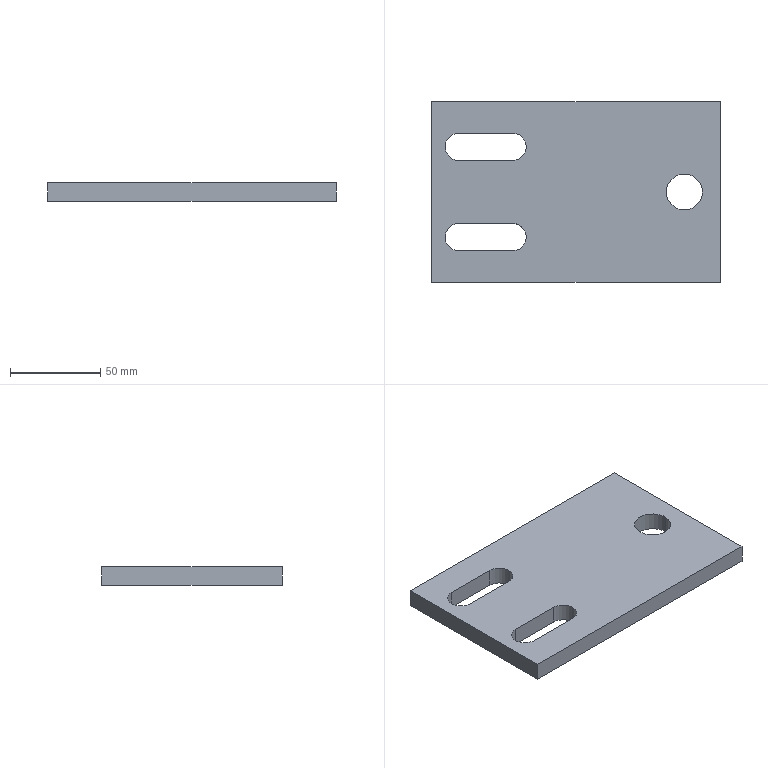Part | SolidWorks | features BaseBody 1 | 1 solid | 18 faces | box 160 x 100 x 10 mm | volume 144324 mm3 | plane 10 | cylinder 8 | commonest cylinder face diameters 15 x6 20 x2
STEP:
#1=CARTESIAN_POINT('',(70.,0.,0.));
#2=VERTEX_POINT('',#1);
#3=CARTESIAN_POINT('',(50.,0.,0.));
#4=VERTEX_POINT('',#3);
#5=CARTESIAN_POINT('',(60.,0.,0.));
#6=DIRECTION('',(0.,0.,-1.));
#7=DIRECTION('',(1.,0.,0.));
#8=AXIS2_PLACEMENT_3D('',#5,#6,#7);
#9=CIRCLE('',#8,10.);
#10=EDGE_CURVE('',#2,#4,#9,.T.);
#11=ORIENTED_EDGE('',*,*,#10,.T.);
#12=CARTESIAN_POINT('',(50.,0.,10.));
#13=VERTEX_POINT('',#12);
#14=CARTESIAN_POINT('',(50.,0.,0.));
#15=DIRECTION('',(0.,0.,1.));
#16=VECTOR('',#15,1000.);
#17=LINE('',#14,#16);
#18=EDGE_CURVE('',#4,#13,#17,.T.);
#19=ORIENTED_EDGE('',*,*,#18,.T.);
#20=CARTESIAN_POINT('',(70.,0.,10.));
#21=VERTEX_POINT('',#20);
#22=CARTESIAN_POINT('',(60.,0.,10.));
#23=DIRECTION('',(0.,0.,-1.));
#24=DIRECTION('',(1.,0.,0.));
#25=AXIS2_PLACEMENT_3D('',#22,#23,#24);
#26=CIRCLE('',#25,10.);
#27=EDGE_CURVE('',#21,#13,#26,.T.);
#28=ORIENTED_EDGE('',*,*,#27,.F.);
#29=CARTESIAN_POINT('',(70.,0.,0.));
#30=DIRECTION('',(0.,0.,1.));
#31=VECTOR('',#30,1000.);
#32=LINE('',#29,#31);
#33=EDGE_CURVE('',#2,#21,#32,.T.);
#34=ORIENTED_EDGE('',*,*,#33,.F.);
#35=EDGE_LOOP('',(#11,#19,#28,#34));
#36=FACE_OUTER_BOUND('',#35,.T.);
#37=CARTESIAN_POINT('',(60.,0.,0.));
#38=DIRECTION('',(0.,0.,1.));
#39=DIRECTION('',(1.,0.,0.));
#40=AXIS2_PLACEMENT_3D('',#37,#38,#39);
#41=CYLINDRICAL_SURFACE('',#40,10.);
#42=ADVANCED_FACE('',(#36),#41,.F.);
#43=CARTESIAN_POINT('',(-72.5,-25.,10.));
#44=VERTEX_POINT('',#43);
#45=CARTESIAN_POINT('',(-65.,-17.5,10.));
#46=VERTEX_POINT('',#45);
#47=CARTESIAN_POINT('',(-65.,-25.,10.));
#48=DIRECTION('',(0.,0.,-1.));
#49=DIRECTION('',(-1.,0.,0.));
#50=AXIS2_PLACEMENT_3D('',#47,#48,#49);
#51=CIRCLE('',#50,7.5);
#52=EDGE_CURVE('',#44,#46,#51,.T.);
#53=ORIENTED_EDGE('',*,*,#52,.F.);
#54=CARTESIAN_POINT('',(-72.5,-25.,0.));
#55=VERTEX_POINT('',#54);
#56=CARTESIAN_POINT('',(-72.5,-25.,10.));
#57=DIRECTION('',(0.,0.,-1.));
#58=VECTOR('',#57,1000.);
#59=LINE('',#56,#58);
#60=EDGE_CURVE('',#44,#55,#59,.T.);
#61=ORIENTED_EDGE('',*,*,#60,.T.);
#62=CARTESIAN_POINT('',(-65.,-17.5,0.));
#63=VERTEX_POINT('',#62);
#64=CARTESIAN_POINT('',(-65.,-25.,0.));
#65=DIRECTION('',(0.,0.,-1.));
#66=DIRECTION('',(-1.,0.,0.));
#67=AXIS2_PLACEMENT_3D('',#64,#65,#66);
#68=CIRCLE('',#67,7.5);
#69=EDGE_CURVE('',#55,#63,#68,.T.);
#70=ORIENTED_EDGE('',*,*,#69,.T.);
#71=CARTESIAN_POINT('',(-65.,-17.5,10.));
#72=DIRECTION('',(0.,0.,1.));
#73=VECTOR('',#72,1000.);
#74=LINE('',#71,#73);
#75=EDGE_CURVE('',#63,#46,#74,.T.);
#76=ORIENTED_EDGE('',*,*,#75,.T.);
#77=EDGE_LOOP('',(#53,#61,#70,#76));
#78=FACE_OUTER_BOUND('',#77,.T.);
#79=CARTESIAN_POINT('',(-65.,-25.,10.));
#80=DIRECTION('',(0.,0.,-1.));
#81=DIRECTION('',(-1.,0.,0.));
#82=AXIS2_PLACEMENT_3D('',#79,#80,#81);
#83=CYLINDRICAL_SURFACE('',#82,7.5);
#84=ADVANCED_FACE('',(#78),#83,.F.);
#85=CARTESIAN_POINT('',(-72.5,25.,10.));
#86=VERTEX_POINT('',#85);
#87=CARTESIAN_POINT('',(-65.,32.5,10.));
#88=VERTEX_POINT('',#87);
#89=CARTESIAN_POINT('',(-65.,25.,10.));
#90=DIRECTION('',(0.,0.,-1.));
#91=DIRECTION('',(-1.,0.,0.));
#92=AXIS2_PLACEMENT_3D('',#89,#90,#91);
#93=CIRCLE('',#92,7.5);
#94=EDGE_CURVE('',#86,#88,#93,.T.);
#95=ORIENTED_EDGE('',*,*,#94,.F.);
#96=CARTESIAN_POINT('',(-72.5,25.,0.));
#97=VERTEX_POINT('',#96);
#98=CARTESIAN_POINT('',(-72.5,25.,10.));
#99=DIRECTION('',(0.,0.,-1.));
#100=VECTOR('',#99,1000.);
#101=LINE('',#98,#100);
#102=EDGE_CURVE('',#86,#97,#101,.T.);
#103=ORIENTED_EDGE('',*,*,#102,.T.);
#104=CARTESIAN_POINT('',(-65.,32.5,0.));
#105=VERTEX_POINT('',#104);
#106=CARTESIAN_POINT('',(-65.,25.,0.));
#107=DIRECTION('',(0.,0.,-1.));
#108=DIRECTION('',(-1.,0.,0.));
#109=AXIS2_PLACEMENT_3D('',#106,#107,#108);
#110=CIRCLE('',#109,7.5);
#111=EDGE_CURVE('',#97,#105,#110,.T.);
#112=ORIENTED_EDGE('',*,*,#111,.T.);
#113=CARTESIAN_POINT('',(-65.,32.5,10.));
#114=DIRECTION('',(0.,0.,1.));
#115=VECTOR('',#114,1000.);
#116=LINE('',#113,#115);
#117=EDGE_CURVE('',#105,#88,#116,.T.);
#118=ORIENTED_EDGE('',*,*,#117,.T.);
#119=EDGE_LOOP('',(#95,#103,#112,#118));
#120=FACE_OUTER_BOUND('',#119,.T.);
#121=CARTESIAN_POINT('',(-65.,25.,10.));
#122=DIRECTION('',(0.,0.,-1.));
#123=DIRECTION('',(-1.,0.,0.));
#124=AXIS2_PLACEMENT_3D('',#121,#122,#123);
#125=CYLINDRICAL_SURFACE('',#124,7.5);
#126=ADVANCED_FACE('',(#120),#125,.F.);
#127=ORIENTED_EDGE('',*,*,#10,.F.);
#128=CARTESIAN_POINT('',(60.,0.,0.));
#129=DIRECTION('',(0.,0.,-1.));
#130=DIRECTION('',(1.,0.,0.));
#131=AXIS2_PLACEMENT_3D('',#128,#129,#130);
#132=CIRCLE('',#131,10.);
#133=EDGE_CURVE('',#4,#2,#132,.T.);
#134=ORIENTED_EDGE('',*,*,#133,.F.);
#135=EDGE_LOOP('',(#127,#134));
#136=FACE_BOUND('',#135,.T.);
#137=CARTESIAN_POINT('',(-35.,-17.5,0.));
#138=VERTEX_POINT('',#137);
#139=CARTESIAN_POINT('',(0.,-17.5,0.));
#140=DIRECTION('',(1.,0.,0.));
#141=VECTOR('',#140,1000.);
#142=LINE('',#139,#141);
#143=EDGE_CURVE('',#63,#138,#142,.T.);
#144=ORIENTED_EDGE('',*,*,#143,.F.);
#145=ORIENTED_EDGE('',*,*,#69,.F.);
#146=CARTESIAN_POINT('',(-65.,-32.5,0.));
#147=VERTEX_POINT('',#146);
#148=CARTESIAN_POINT('',(-65.,-25.,0.));
#149=DIRECTION('',(0.,0.,-1.));
#150=DIRECTION('',(-1.,0.,0.));
#151=AXIS2_PLACEMENT_3D('',#148,#149,#150);
#152=CIRCLE('',#151,7.5);
#153=EDGE_CURVE('',#147,#55,#152,.T.);
#154=ORIENTED_EDGE('',*,*,#153,.F.);
#155=CARTESIAN_POINT('',(-35.,-32.5,0.));
#156=VERTEX_POINT('',#155);
#157=CARTESIAN_POINT('',(0.,-32.5,0.));
#158=DIRECTION('',(-1.,0.,0.));
#159=VECTOR('',#158,1000.);
#160=LINE('',#157,#159);
#161=EDGE_CURVE('',#156,#147,#160,.T.);
#162=ORIENTED_EDGE('',*,*,#161,.F.);
#163=CARTESIAN_POINT('',(-35.,-25.,0.));
#164=DIRECTION('',(0.,0.,-1.));
#165=DIRECTION('',(-1.,0.,0.));
#166=AXIS2_PLACEMENT_3D('',#163,#164,#165);
#167=CIRCLE('',#166,7.5);
#168=EDGE_CURVE('',#138,#156,#167,.T.);
#169=ORIENTED_EDGE('',*,*,#168,.F.);
#170=EDGE_LOOP('',(#144,#145,#154,#162,#169));
#171=FACE_BOUND('',#170,.T.);
#172=CARTESIAN_POINT('',(-35.,32.5,0.));
#173=VERTEX_POINT('',#172);
#174=CARTESIAN_POINT('',(0.,32.5,0.));
#175=DIRECTION('',(1.,0.,0.));
#176=VECTOR('',#175,1000.);
#177=LINE('',#174,#176);
#178=EDGE_CURVE('',#105,#173,#177,.T.);
#179=ORIENTED_EDGE('',*,*,#178,.F.);
#180=ORIENTED_EDGE('',*,*,#111,.F.);
#181=CARTESIAN_POINT('',(-65.,17.5,0.));
#182=VERTEX_POINT('',#181);
#183=CARTESIAN_POINT('',(-65.,25.,0.));
#184=DIRECTION('',(0.,0.,-1.));
#185=DIRECTION('',(-1.,0.,0.));
#186=AXIS2_PLACEMENT_3D('',#183,#184,#185);
#187=CIRCLE('',#186,7.5);
#188=EDGE_CURVE('',#182,#97,#187,.T.);
#189=ORIENTED_EDGE('',*,*,#188,.F.);
#190=CARTESIAN_POINT('',(-35.,17.5,0.));
#191=VERTEX_POINT('',#190);
#192=CARTESIAN_POINT('',(0.,17.5,0.));
#193=DIRECTION('',(-1.,0.,0.));
#194=VECTOR('',#193,1000.);
#195=LINE('',#192,#194);
#196=EDGE_CURVE('',#191,#182,#195,.T.);
#197=ORIENTED_EDGE('',*,*,#196,.F.);
#198=CARTESIAN_POINT('',(-35.,25.,0.));
#199=DIRECTION('',(0.,0.,-1.));
#200=DIRECTION('',(-1.,0.,0.));
#201=AXIS2_PLACEMENT_3D('',#198,#199,#200);
#202=CIRCLE('',#201,7.5);
#203=EDGE_CURVE('',#173,#191,#202,.T.);
#204=ORIENTED_EDGE('',*,*,#203,.F.);
#205=EDGE_LOOP('',(#179,#180,#189,#197,#204));
#206=FACE_BOUND('',#205,.T.);
#207=CARTESIAN_POINT('',(80.,-50.,0.));
#208=VERTEX_POINT('',#207);
#209=CARTESIAN_POINT('',(80.,50.,0.));
#210=VERTEX_POINT('',#209);
#211=CARTESIAN_POINT('',(80.,0.,0.));
#212=DIRECTION('',(0.,1.,0.));
#213=VECTOR('',#212,1000.);
#214=LINE('',#211,#213);
#215=EDGE_CURVE('',#208,#210,#214,.T.);
#216=ORIENTED_EDGE('',*,*,#215,.F.);
#217=CARTESIAN_POINT('',(-80.,-50.,0.));
#218=VERTEX_POINT('',#217);
#219=CARTESIAN_POINT('',(0.,-50.,0.));
#220=DIRECTION('',(1.,0.,0.));
#221=VECTOR('',#220,1000.);
#222=LINE('',#219,#221);
#223=EDGE_CURVE('',#218,#208,#222,.T.);
#224=ORIENTED_EDGE('',*,*,#223,.F.);
#225=CARTESIAN_POINT('',(-80.,50.,0.));
#226=VERTEX_POINT('',#225);
#227=CARTESIAN_POINT('',(-80.,0.,0.));
#228=DIRECTION('',(0.,-1.,0.));
#229=VECTOR('',#228,1000.);
#230=LINE('',#227,#229);
#231=EDGE_CURVE('',#226,#218,#230,.T.);
#232=ORIENTED_EDGE('',*,*,#231,.F.);
#233=CARTESIAN_POINT('',(0.,50.,0.));
#234=DIRECTION('',(-1.,0.,0.));
#235=VECTOR('',#234,1000.);
#236=LINE('',#233,#235);
#237=EDGE_CURVE('',#210,#226,#236,.T.);
#238=ORIENTED_EDGE('',*,*,#237,.F.);
#239=EDGE_LOOP('',(#216,#224,#232,#238));
#240=FACE_OUTER_BOUND('',#239,.T.);
#241=CARTESIAN_POINT('',(0.,0.,0.));
#242=DIRECTION('',(0.,0.,1.));
#243=DIRECTION('',(1.,0.,0.));
#244=AXIS2_PLACEMENT_3D('',#241,#242,#243);
#245=PLANE('',#244);
#246=ADVANCED_FACE('',(#136,#171,#206,#240),#245,.F.);
#247=ORIENTED_EDGE('',*,*,#18,.F.);
#248=ORIENTED_EDGE('',*,*,#133,.T.);
#249=ORIENTED_EDGE('',*,*,#33,.T.);
#250=CARTESIAN_POINT('',(60.,0.,10.));
#251=DIRECTION('',(0.,0.,-1.));
#252=DIRECTION('',(1.,0.,0.));
#253=AXIS2_PLACEMENT_3D('',#250,#251,#252);
#254=CIRCLE('',#253,10.);
#255=EDGE_CURVE('',#13,#21,#254,.T.);
#256=ORIENTED_EDGE('',*,*,#255,.F.);
#257=EDGE_LOOP('',(#247,#248,#249,#256));
#258=FACE_OUTER_BOUND('',#257,.T.);
#259=CARTESIAN_POINT('',(60.,0.,0.));
#260=DIRECTION('',(0.,0.,1.));
#261=DIRECTION('',(1.,0.,0.));
#262=AXIS2_PLACEMENT_3D('',#259,#260,#261);
#263=CYLINDRICAL_SURFACE('',#262,10.);
#264=ADVANCED_FACE('',(#258),#263,.F.);
#265=CARTESIAN_POINT('',(-35.,-17.5,10.));
#266=VERTEX_POINT('',#265);
#267=CARTESIAN_POINT('',(-35.,-17.5,10.));
#268=DIRECTION('',(0.,0.,1.));
#269=VECTOR('',#268,1000.);
#270=LINE('',#267,#269);
#271=EDGE_CURVE('',#138,#266,#270,.T.);
#272=ORIENTED_EDGE('',*,*,#271,.F.);
#273=ORIENTED_EDGE('',*,*,#168,.T.);
#274=CARTESIAN_POINT('',(-35.,-32.5,10.));
#275=VERTEX_POINT('',#274);
#276=CARTESIAN_POINT('',(-35.,-32.5,10.));
#277=DIRECTION('',(0.,0.,-1.));
#278=VECTOR('',#277,1000.);
#279=LINE('',#276,#278);
#280=EDGE_CURVE('',#275,#156,#279,.T.);
#281=ORIENTED_EDGE('',*,*,#280,.F.);
#282=CARTESIAN_POINT('',(-35.,-25.,10.));
#283=DIRECTION('',(0.,0.,-1.));
#284=DIRECTION('',(-1.,0.,0.));
#285=AXIS2_PLACEMENT_3D('',#282,#283,#284);
#286=CIRCLE('',#285,7.5);
#287=EDGE_CURVE('',#266,#275,#286,.T.);
#288=ORIENTED_EDGE('',*,*,#287,.F.);
#289=EDGE_LOOP('',(#272,#273,#281,#288));
#290=FACE_OUTER_BOUND('',#289,.T.);
#291=CARTESIAN_POINT('',(-35.,-25.,10.));
#292=DIRECTION('',(0.,0.,-1.));
#293=DIRECTION('',(-1.,0.,0.));
#294=AXIS2_PLACEMENT_3D('',#291,#292,#293);
#295=CYLINDRICAL_SURFACE('',#294,7.5);
#296=ADVANCED_FACE('',(#290),#295,.F.);
#297=ORIENTED_EDGE('',*,*,#75,.F.);
#298=ORIENTED_EDGE('',*,*,#143,.T.);
#299=ORIENTED_EDGE('',*,*,#271,.T.);
#300=CARTESIAN_POINT('',(-65.,-17.5,10.));
#301=DIRECTION('',(1.,0.,0.));
#302=VECTOR('',#301,1000.);
#303=LINE('',#300,#302);
#304=EDGE_CURVE('',#46,#266,#303,.T.);
#305=ORIENTED_EDGE('',*,*,#304,.F.);
#306=EDGE_LOOP('',(#297,#298,#299,#305));
#307=FACE_OUTER_BOUND('',#306,.T.);
#308=CARTESIAN_POINT('',(-65.,-17.5,10.));
#309=DIRECTION('',(0.,1.,0.));
#310=DIRECTION('',(0.,0.,1.));
#311=AXIS2_PLACEMENT_3D('',#308,#309,#310);
#312=PLANE('',#311);
#313=ADVANCED_FACE('',(#307),#312,.F.);
#314=ORIENTED_EDGE('',*,*,#60,.F.);
#315=CARTESIAN_POINT('',(-65.,-32.5,10.));
#316=VERTEX_POINT('',#315);
#317=CARTESIAN_POINT('',(-65.,-25.,10.));
#318=DIRECTION('',(0.,0.,-1.));
#319=DIRECTION('',(-1.,0.,0.));
#320=AXIS2_PLACEMENT_3D('',#317,#318,#319);
#321=CIRCLE('',#320,7.5);
#322=EDGE_CURVE('',#316,#44,#321,.T.);
#323=ORIENTED_EDGE('',*,*,#322,.F.);
#324=CARTESIAN_POINT('',(-65.,-32.5,10.));
#325=DIRECTION('',(0.,0.,1.));
#326=VECTOR('',#325,1000.);
#327=LINE('',#324,#326);
#328=EDGE_CURVE('',#147,#316,#327,.T.);
#329=ORIENTED_EDGE('',*,*,#328,.F.);
#330=ORIENTED_EDGE('',*,*,#153,.T.);
#331=EDGE_LOOP('',(#314,#323,#329,#330));
#332=FACE_OUTER_BOUND('',#331,.T.);
#333=CARTESIAN_POINT('',(-65.,-25.,10.));
#334=DIRECTION('',(0.,0.,-1.));
#335=DIRECTION('',(-1.,0.,0.));
#336=AXIS2_PLACEMENT_3D('',#333,#334,#335);
#337=CYLINDRICAL_SURFACE('',#336,7.5);
#338=ADVANCED_FACE('',(#332),#337,.F.);
#339=ORIENTED_EDGE('',*,*,#280,.T.);
#340=ORIENTED_EDGE('',*,*,#161,.T.);
#341=ORIENTED_EDGE('',*,*,#328,.T.);
#342=CARTESIAN_POINT('',(-35.,-32.5,10.));
#343=DIRECTION('',(-1.,0.,0.));
#344=VECTOR('',#343,1000.);
#345=LINE('',#342,#344);
#346=EDGE_CURVE('',#275,#316,#345,.T.);
#347=ORIENTED_EDGE('',*,*,#346,.F.);
#348=EDGE_LOOP('',(#339,#340,#341,#347));
#349=FACE_OUTER_BOUND('',#348,.T.);
#350=CARTESIAN_POINT('',(-35.,-32.5,10.));
#351=DIRECTION('',(0.,-1.,0.));
#352=DIRECTION('',(0.,0.,-1.));
#353=AXIS2_PLACEMENT_3D('',#350,#351,#352);
#354=PLANE('',#353);
#355=ADVANCED_FACE('',(#349),#354,.F.);
#356=CARTESIAN_POINT('',(-35.,32.5,10.));
#357=VERTEX_POINT('',#356);
#358=CARTESIAN_POINT('',(-35.,32.5,10.));
#359=DIRECTION('',(0.,0.,1.));
#360=VECTOR('',#359,1000.);
#361=LINE('',#358,#360);
#362=EDGE_CURVE('',#173,#357,#361,.T.);
#363=ORIENTED_EDGE('',*,*,#362,.F.);
#364=ORIENTED_EDGE('',*,*,#203,.T.);
#365=CARTESIAN_POINT('',(-35.,17.5,10.));
#366=VERTEX_POINT('',#365);
#367=CARTESIAN_POINT('',(-35.,17.5,10.));
#368=DIRECTION('',(0.,0.,-1.));
#369=VECTOR('',#368,1000.);
#370=LINE('',#367,#369);
#371=EDGE_CURVE('',#366,#191,#370,.T.);
#372=ORIENTED_EDGE('',*,*,#371,.F.);
#373=CARTESIAN_POINT('',(-35.,25.,10.));
#374=DIRECTION('',(0.,0.,-1.));
#375=DIRECTION('',(-1.,0.,0.));
#376=AXIS2_PLACEMENT_3D('',#373,#374,#375);
#377=CIRCLE('',#376,7.5);
#378=EDGE_CURVE('',#357,#366,#377,.T.);
#379=ORIENTED_EDGE('',*,*,#378,.F.);
#380=EDGE_LOOP('',(#363,#364,#372,#379));
#381=FACE_OUTER_BOUND('',#380,.T.);
#382=CARTESIAN_POINT('',(-35.,25.,10.));
#383=DIRECTION('',(0.,0.,-1.));
#384=DIRECTION('',(-1.,0.,0.));
#385=AXIS2_PLACEMENT_3D('',#382,#383,#384);
#386=CYLINDRICAL_SURFACE('',#385,7.5);
#387=ADVANCED_FACE('',(#381),#386,.F.);
#388=ORIENTED_EDGE('',*,*,#117,.F.);
#389=ORIENTED_EDGE('',*,*,#178,.T.);
#390=ORIENTED_EDGE('',*,*,#362,.T.);
#391=CARTESIAN_POINT('',(-65.,32.5,10.));
#392=DIRECTION('',(1.,0.,0.));
#393=VECTOR('',#392,1000.);
#394=LINE('',#391,#393);
#395=EDGE_CURVE('',#88,#357,#394,.T.);
#396=ORIENTED_EDGE('',*,*,#395,.F.);
#397=EDGE_LOOP('',(#388,#389,#390,#396));
#398=FACE_OUTER_BOUND('',#397,.T.);
#399=CARTESIAN_POINT('',(-65.,32.5,10.));
#400=DIRECTION('',(0.,1.,0.));
#401=DIRECTION('',(0.,0.,1.));
#402=AXIS2_PLACEMENT_3D('',#399,#400,#401);
#403=PLANE('',#402);
#404=ADVANCED_FACE('',(#398),#403,.F.);
#405=ORIENTED_EDGE('',*,*,#102,.F.);
#406=CARTESIAN_POINT('',(-65.,17.5,10.));
#407=VERTEX_POINT('',#406);
#408=CARTESIAN_POINT('',(-65.,25.,10.));
#409=DIRECTION('',(0.,0.,-1.));
#410=DIRECTION('',(-1.,0.,0.));
#411=AXIS2_PLACEMENT_3D('',#408,#409,#410);
#412=CIRCLE('',#411,7.5);
#413=EDGE_CURVE('',#407,#86,#412,.T.);
#414=ORIENTED_EDGE('',*,*,#413,.F.);
#415=CARTESIAN_POINT('',(-65.,17.5,10.));
#416=DIRECTION('',(0.,0.,1.));
#417=VECTOR('',#416,1000.);
#418=LINE('',#415,#417);
#419=EDGE_CURVE('',#182,#407,#418,.T.);
#420=ORIENTED_EDGE('',*,*,#419,.F.);
#421=ORIENTED_EDGE('',*,*,#188,.T.);
#422=EDGE_LOOP('',(#405,#414,#420,#421));
#423=FACE_OUTER_BOUND('',#422,.T.);
#424=CARTESIAN_POINT('',(-65.,25.,10.));
#425=DIRECTION('',(0.,0.,-1.));
#426=DIRECTION('',(-1.,0.,0.));
#427=AXIS2_PLACEMENT_3D('',#424,#425,#426);
#428=CYLINDRICAL_SURFACE('',#427,7.5);
#429=ADVANCED_FACE('',(#423),#428,.F.);
#430=ORIENTED_EDGE('',*,*,#371,.T.);
#431=ORIENTED_EDGE('',*,*,#196,.T.);
#432=ORIENTED_EDGE('',*,*,#419,.T.);
#433=CARTESIAN_POINT('',(-35.,17.5,10.));
#434=DIRECTION('',(-1.,0.,0.));
#435=VECTOR('',#434,1000.);
#436=LINE('',#433,#435);
#437=EDGE_CURVE('',#366,#407,#436,.T.);
#438=ORIENTED_EDGE('',*,*,#437,.F.);
#439=EDGE_LOOP('',(#430,#431,#432,#438));
#440=FACE_OUTER_BOUND('',#439,.T.);
#441=CARTESIAN_POINT('',(-35.,17.5,10.));
#442=DIRECTION('',(0.,-1.,0.));
#443=DIRECTION('',(1.,0.,0.));
#444=AXIS2_PLACEMENT_3D('',#441,#442,#443);
#445=PLANE('',#444);
#446=ADVANCED_FACE('',(#440),#445,.F.);
#447=ORIENTED_EDGE('',*,*,#237,.T.);
#448=CARTESIAN_POINT('',(-80.,50.,10.));
#449=VERTEX_POINT('',#448);
#450=CARTESIAN_POINT('',(-80.,50.,0.));
#451=DIRECTION('',(0.,0.,1.));
#452=VECTOR('',#451,1000.);
#453=LINE('',#450,#452);
#454=EDGE_CURVE('',#226,#449,#453,.T.);
#455=ORIENTED_EDGE('',*,*,#454,.T.);
#456=CARTESIAN_POINT('',(80.,50.,10.));
#457=VERTEX_POINT('',#456);
#458=CARTESIAN_POINT('',(-80.,50.,10.));
#459=DIRECTION('',(1.,0.,0.));
#460=VECTOR('',#459,1000.);
#461=LINE('',#458,#460);
#462=EDGE_CURVE('',#449,#457,#461,.T.);
#463=ORIENTED_EDGE('',*,*,#462,.T.);
#464=CARTESIAN_POINT('',(80.,50.,0.));
#465=DIRECTION('',(0.,0.,-1.));
#466=VECTOR('',#465,1000.);
#467=LINE('',#464,#466);
#468=EDGE_CURVE('',#457,#210,#467,.T.);
#469=ORIENTED_EDGE('',*,*,#468,.T.);
#470=EDGE_LOOP('',(#447,#455,#463,#469));
#471=FACE_OUTER_BOUND('',#470,.T.);
#472=CARTESIAN_POINT('',(-80.,50.,0.));
#473=DIRECTION('',(0.,1.,0.));
#474=DIRECTION('',(0.,0.,1.));
#475=AXIS2_PLACEMENT_3D('',#472,#473,#474);
#476=PLANE('',#475);
#477=ADVANCED_FACE('',(#471),#476,.T.);
#478=ORIENTED_EDGE('',*,*,#215,.T.);
#479=ORIENTED_EDGE('',*,*,#468,.F.);
#480=CARTESIAN_POINT('',(80.,-50.,10.));
#481=VERTEX_POINT('',#480);
#482=CARTESIAN_POINT('',(80.,50.,10.));
#483=DIRECTION('',(0.,-1.,0.));
#484=VECTOR('',#483,1000.);
#485=LINE('',#482,#484);
#486=EDGE_CURVE('',#457,#481,#485,.T.);
#487=ORIENTED_EDGE('',*,*,#486,.T.);
#488=CARTESIAN_POINT('',(80.,-50.,0.));
#489=DIRECTION('',(0.,0.,-1.));
#490=VECTOR('',#489,1000.);
#491=LINE('',#488,#490);
#492=EDGE_CURVE('',#481,#208,#491,.T.);
#493=ORIENTED_EDGE('',*,*,#492,.T.);
#494=EDGE_LOOP('',(#478,#479,#487,#493));
#495=FACE_OUTER_BOUND('',#494,.T.);
#496=CARTESIAN_POINT('',(80.,50.,0.));
#497=DIRECTION('',(1.,0.,0.));
#498=DIRECTION('',(0.,0.,-1.));
#499=AXIS2_PLACEMENT_3D('',#496,#497,#498);
#500=PLANE('',#499);
#501=ADVANCED_FACE('',(#495),#500,.T.);
#502=ORIENTED_EDGE('',*,*,#223,.T.);
#503=ORIENTED_EDGE('',*,*,#492,.F.);
#504=CARTESIAN_POINT('',(-80.,-50.,10.));
#505=VERTEX_POINT('',#504);
#506=CARTESIAN_POINT('',(80.,-50.,10.));
#507=DIRECTION('',(-1.,0.,0.));
#508=VECTOR('',#507,1000.);
#509=LINE('',#506,#508);
#510=EDGE_CURVE('',#481,#505,#509,.T.);
#511=ORIENTED_EDGE('',*,*,#510,.T.);
#512=CARTESIAN_POINT('',(-80.,-50.,0.));
#513=DIRECTION('',(0.,0.,-1.));
#514=VECTOR('',#513,1000.);
#515=LINE('',#512,#514);
#516=EDGE_CURVE('',#505,#218,#515,.T.);
#517=ORIENTED_EDGE('',*,*,#516,.T.);
#518=EDGE_LOOP('',(#502,#503,#511,#517));
#519=FACE_OUTER_BOUND('',#518,.T.);
#520=CARTESIAN_POINT('',(80.,-50.,0.));
#521=DIRECTION('',(0.,-1.,0.));
#522=DIRECTION('',(1.,0.,0.));
#523=AXIS2_PLACEMENT_3D('',#520,#521,#522);
#524=PLANE('',#523);
#525=ADVANCED_FACE('',(#519),#524,.T.);
#526=ORIENTED_EDGE('',*,*,#231,.T.);
#527=ORIENTED_EDGE('',*,*,#516,.F.);
#528=CARTESIAN_POINT('',(-80.,-50.,10.));
#529=DIRECTION('',(0.,1.,0.));
#530=VECTOR('',#529,1000.);
#531=LINE('',#528,#530);
#532=EDGE_CURVE('',#505,#449,#531,.T.);
#533=ORIENTED_EDGE('',*,*,#532,.T.);
#534=ORIENTED_EDGE('',*,*,#454,.F.);
#535=EDGE_LOOP('',(#526,#527,#533,#534));
#536=FACE_OUTER_BOUND('',#535,.T.);
#537=CARTESIAN_POINT('',(-80.,-50.,0.));
#538=DIRECTION('',(-1.,0.,0.));
#539=DIRECTION('',(0.,-1.,0.));
#540=AXIS2_PLACEMENT_3D('',#537,#538,#539);
#541=PLANE('',#540);
#542=ADVANCED_FACE('',(#536),#541,.T.);
#543=ORIENTED_EDGE('',*,*,#27,.T.);
#544=ORIENTED_EDGE('',*,*,#255,.T.);
#545=EDGE_LOOP('',(#543,#544));
#546=FACE_BOUND('',#545,.T.);
#547=ORIENTED_EDGE('',*,*,#322,.T.);
#548=ORIENTED_EDGE('',*,*,#52,.T.);
#549=ORIENTED_EDGE('',*,*,#304,.T.);
#550=ORIENTED_EDGE('',*,*,#287,.T.);
#551=ORIENTED_EDGE('',*,*,#346,.T.);
#552=EDGE_LOOP('',(#547,#548,#549,#550,#551));
#553=FACE_BOUND('',#552,.T.);
#554=ORIENTED_EDGE('',*,*,#413,.T.);
#555=ORIENTED_EDGE('',*,*,#94,.T.);
#556=ORIENTED_EDGE('',*,*,#395,.T.);
#557=ORIENTED_EDGE('',*,*,#378,.T.);
#558=ORIENTED_EDGE('',*,*,#437,.T.);
#559=EDGE_LOOP('',(#554,#555,#556,#557,#558));
#560=FACE_BOUND('',#559,.T.);
#561=ORIENTED_EDGE('',*,*,#532,.F.);
#562=ORIENTED_EDGE('',*,*,#510,.F.);
#563=ORIENTED_EDGE('',*,*,#486,.F.);
#564=ORIENTED_EDGE('',*,*,#462,.F.);
#565=EDGE_LOOP('',(#561,#562,#563,#564));
#566=FACE_OUTER_BOUND('',#565,.T.);
#567=CARTESIAN_POINT('',(0.,0.,10.));
#568=DIRECTION('',(0.,0.,1.));
#569=DIRECTION('',(1.,0.,0.));
#570=AXIS2_PLACEMENT_3D('',#567,#568,#569);
#571=PLANE('',#570);
#572=ADVANCED_FACE('',(#546,#553,#560,#566),#571,.T.);
#573=CLOSED_SHELL('',(#42,#84,#126,#246,#264,#296,#313,#338,#355,#387,#404,#429,#446,#477,#501,#525,#542,#572));
#574=MANIFOLD_SOLID_BREP('',#573);
#575=CARTESIAN_POINT('',(0.,0.,0.));
#576=DIRECTION('',(0.,0.,1.));
#577=DIRECTION('',(1.,0.,0.));
#578=AXIS2_PLACEMENT_3D('',#575,#576,#577);
#579=(LENGTH_UNIT()NAMED_UNIT(*)SI_UNIT(.MILLI.,.METRE.));
#580=UNCERTAINTY_MEASURE_WITH_UNIT(LENGTH_MEASURE(0.00001),#579,'','');
#581=(NAMED_UNIT(*)PLANE_ANGLE_UNIT()SI_UNIT($,.RADIAN.));
#582=(NAMED_UNIT(*)SI_UNIT($,.STERADIAN.)SOLID_ANGLE_UNIT());
#583=(GEOMETRIC_REPRESENTATION_CONTEXT(3)GLOBAL_UNCERTAINTY_ASSIGNED_CONTEXT((#580))GLOBAL_UNIT_ASSIGNED_CONTEXT((#579,#581,#582))REPRESENTATION_CONTEXT('',''));
#584=ADVANCED_BREP_SHAPE_REPRESENTATION('',(#574,#578),#583);